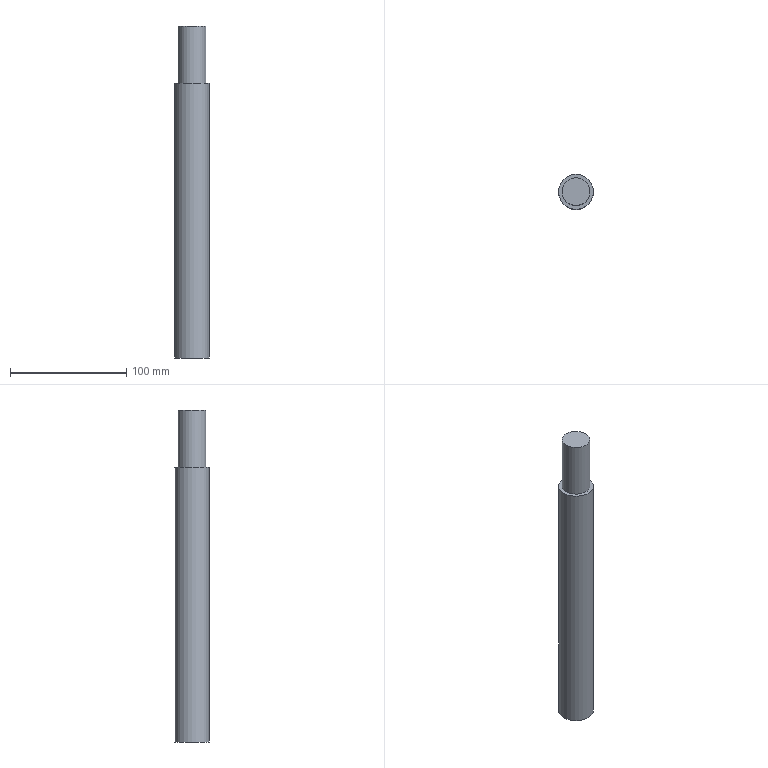Part | NX | features solid 2 | 1 solid | 5 faces | box 30 x 30 x 285 mm | volume 188986 mm3 | plane 3 | cylinder 2 | commonest cylinder face diameters 24 x1 30 x1
STEP:
#1=CARTESIAN_POINT('',(-65.,-60.,-49.));
#2=VERTEX_POINT('',#1);
#3=CARTESIAN_POINT('',(-80.,-60.,-49.));
#4=DIRECTION('',(0.,0.,1.));
#5=DIRECTION('',(1.,0.,0.));
#6=AXIS2_PLACEMENT_3D('',#3,#4,#5);
#7=CIRCLE('',#6,15.);
#8=EDGE_CURVE('',#2,#2,#7,.T.);
#9=ORIENTED_EDGE('',*,*,#8,.T.);
#10=EDGE_LOOP('',(#9));
#11=FACE_BOUND('',#10,.T.);
#12=CARTESIAN_POINT('',(-92.,-60.,-49.));
#13=VERTEX_POINT('',#12);
#14=CARTESIAN_POINT('',(-80.,-60.,-49.));
#15=DIRECTION('',(0.,0.,-1.));
#16=DIRECTION('',(-1.,0.,0.));
#17=AXIS2_PLACEMENT_3D('',#14,#15,#16);
#18=CIRCLE('',#17,12.);
#19=EDGE_CURVE('',#13,#13,#18,.F.);
#20=ORIENTED_EDGE('',*,*,#19,.F.);
#21=EDGE_LOOP('',(#20));
#22=FACE_BOUND('',#21,.T.);
#23=CARTESIAN_POINT('',(-80.,-60.,-49.));
#24=DIRECTION('',(0.,0.,1.));
#25=DIRECTION('',(1.,0.,0.));
#26=AXIS2_PLACEMENT_3D('',#23,#24,#25);
#27=PLANE('',#26);
#28=ADVANCED_FACE('',(#11,#22),#27,.T.);
#29=ORIENTED_EDGE('',*,*,#8,.F.);
#30=EDGE_LOOP('',(#29));
#31=FACE_BOUND('',#30,.T.);
#32=CARTESIAN_POINT('',(-65.,-60.,-285.));
#33=VERTEX_POINT('',#32);
#34=CARTESIAN_POINT('',(-80.,-60.,-285.));
#35=DIRECTION('',(0.,0.,1.));
#36=DIRECTION('',(1.,0.,0.));
#37=AXIS2_PLACEMENT_3D('',#34,#35,#36);
#38=CIRCLE('',#37,15.);
#39=EDGE_CURVE('',#33,#33,#38,.T.);
#40=ORIENTED_EDGE('',*,*,#39,.T.);
#41=EDGE_LOOP('',(#40));
#42=FACE_BOUND('',#41,.T.);
#43=CARTESIAN_POINT('',(-80.,-60.,-49.));
#44=DIRECTION('',(0.,0.,-1.));
#45=DIRECTION('',(-1.,0.,0.));
#46=AXIS2_PLACEMENT_3D('',#43,#44,#45);
#47=CYLINDRICAL_SURFACE('',#46,15.);
#48=ADVANCED_FACE('',(#31,#42),#47,.T.);
#49=ORIENTED_EDGE('',*,*,#39,.F.);
#50=EDGE_LOOP('',(#49));
#51=FACE_BOUND('',#50,.T.);
#52=CARTESIAN_POINT('',(-80.,-60.,-285.));
#53=DIRECTION('',(0.,0.,1.));
#54=DIRECTION('',(1.,0.,0.));
#55=AXIS2_PLACEMENT_3D('',#52,#53,#54);
#56=PLANE('',#55);
#57=ADVANCED_FACE('',(#51),#56,.F.);
#58=ORIENTED_EDGE('',*,*,#19,.T.);
#59=EDGE_LOOP('',(#58));
#60=FACE_BOUND('',#59,.T.);
#61=CARTESIAN_POINT('',(-92.,-60.,0.));
#62=VERTEX_POINT('',#61);
#63=CARTESIAN_POINT('',(-80.,-60.,0.));
#64=DIRECTION('',(0.,0.,-1.));
#65=DIRECTION('',(-1.,0.,0.));
#66=AXIS2_PLACEMENT_3D('',#63,#64,#65);
#67=CIRCLE('',#66,12.);
#68=EDGE_CURVE('',#62,#62,#67,.F.);
#69=ORIENTED_EDGE('',*,*,#68,.F.);
#70=EDGE_LOOP('',(#69));
#71=FACE_BOUND('',#70,.T.);
#72=CARTESIAN_POINT('',(-80.,-60.,0.));
#73=DIRECTION('',(0.,0.,-1.));
#74=DIRECTION('',(-1.,0.,0.));
#75=AXIS2_PLACEMENT_3D('',#72,#73,#74);
#76=CYLINDRICAL_SURFACE('',#75,12.);
#77=ADVANCED_FACE('',(#60,#71),#76,.T.);
#78=ORIENTED_EDGE('',*,*,#68,.T.);
#79=EDGE_LOOP('',(#78));
#80=FACE_BOUND('',#79,.T.);
#81=CARTESIAN_POINT('',(-80.,-60.,0.));
#82=DIRECTION('',(0.,0.,1.));
#83=DIRECTION('',(1.,0.,0.));
#84=AXIS2_PLACEMENT_3D('',#81,#82,#83);
#85=PLANE('',#84);
#86=ADVANCED_FACE('',(#80),#85,.T.);
#87=CLOSED_SHELL('',(#28,#48,#57,#77,#86));
#88=MANIFOLD_SOLID_BREP('',#87);
#89=(LENGTH_UNIT()NAMED_UNIT(*)SI_UNIT(.MILLI.,.METRE.));
#90=UNCERTAINTY_MEASURE_WITH_UNIT(LENGTH_MEASURE(0.00001),#89,'','');
#91=(NAMED_UNIT(*)PLANE_ANGLE_UNIT()SI_UNIT($,.RADIAN.));
#92=(NAMED_UNIT(*)SI_UNIT($,.STERADIAN.)SOLID_ANGLE_UNIT());
#93=(GEOMETRIC_REPRESENTATION_CONTEXT(3)GLOBAL_UNCERTAINTY_ASSIGNED_CONTEXT((#90))GLOBAL_UNIT_ASSIGNED_CONTEXT((#89,#91,#92))REPRESENTATION_CONTEXT('',''));
#94=ADVANCED_BREP_SHAPE_REPRESENTATION('',(#88),#93);